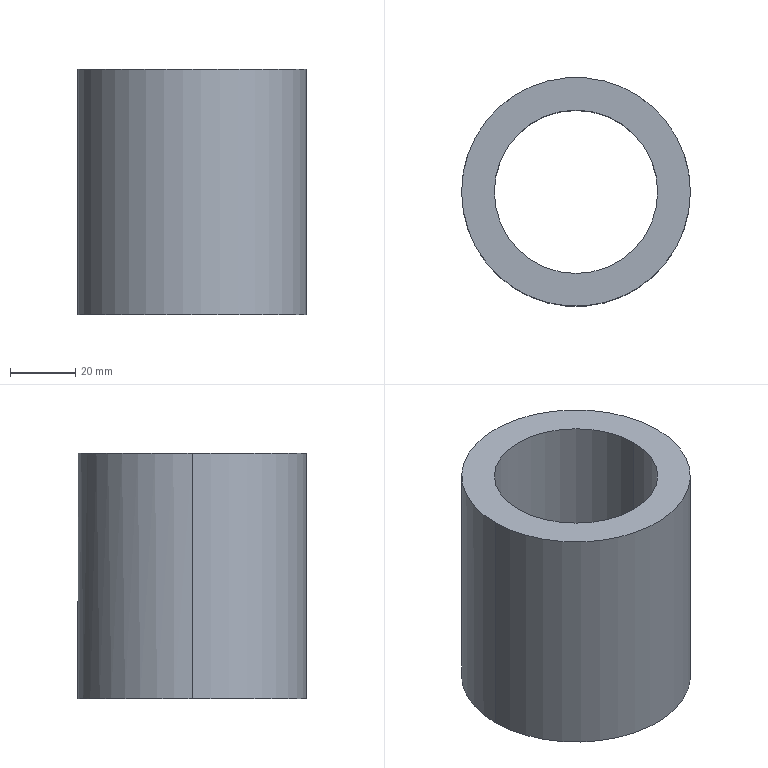Part | Creo | 1 solid | 10 faces | box 70 x 70 x 75 mm | volume 141338 mm3 | cylinder 4 | torus 4 | plane 2 | commonest cylinder face diameters 50 x2 70 x2
STEP:
#1=CARTESIAN_POINT('',(0.,0.,0.));
#2=DIRECTION('',(0.,0.,1.));
#3=DIRECTION('',(1.,0.,0.));
#4=AXIS2_PLACEMENT_3D('',#1,#2,#3);
#5=CARTESIAN_POINT('',(461.101,252.373,51.559));
#6=VERTEX_POINT('',#5);
#7=CARTESIAN_POINT('',(391.101,252.373,51.559));
#8=VERTEX_POINT('',#7);
#9=CARTESIAN_POINT('',(426.101,252.373,51.559));
#10=DIRECTION('',(0.,0.,1.));
#11=DIRECTION('',(1.,0.,0.));
#12=AXIS2_PLACEMENT_3D('',#9,#10,#11);
#13=CIRCLE('',#12,35.);
#14=EDGE_CURVE('',#6,#8,#13,.T.);
#15=ORIENTED_EDGE('',*,*,#14,.F.);
#16=CARTESIAN_POINT('',(426.101,252.373,51.559));
#17=DIRECTION('',(0.,0.,1.));
#18=DIRECTION('',(-1.,0.,0.));
#19=AXIS2_PLACEMENT_3D('',#16,#17,#18);
#20=CIRCLE('',#19,35.);
#21=EDGE_CURVE('',#8,#6,#20,.T.);
#22=ORIENTED_EDGE('',*,*,#21,.F.);
#23=EDGE_LOOP('',(#15,#22));
#24=FACE_OUTER_BOUND('',#23,.F.);
#25=CARTESIAN_POINT('',(451.101,252.373,51.559));
#26=VERTEX_POINT('',#25);
#27=CARTESIAN_POINT('',(401.101,252.373,51.559));
#28=VERTEX_POINT('',#27);
#29=CARTESIAN_POINT('',(426.101,252.373,51.559));
#30=DIRECTION('',(0.,0.,-1.));
#31=DIRECTION('',(1.,0.,0.));
#32=AXIS2_PLACEMENT_3D('',#29,#30,#31);
#33=CIRCLE('',#32,25.);
#34=EDGE_CURVE('',#26,#28,#33,.T.);
#35=ORIENTED_EDGE('',*,*,#34,.F.);
#36=CARTESIAN_POINT('',(426.101,252.373,51.559));
#37=DIRECTION('',(0.,0.,-1.));
#38=DIRECTION('',(-1.,0.,0.));
#39=AXIS2_PLACEMENT_3D('',#36,#37,#38);
#40=CIRCLE('',#39,25.);
#41=EDGE_CURVE('',#28,#26,#40,.T.);
#42=ORIENTED_EDGE('',*,*,#41,.F.);
#43=EDGE_LOOP('',(#35,#42));
#44=FACE_BOUND('',#43,.F.);
#45=CARTESIAN_POINT('',(387.842,227.873,51.559));
#46=DIRECTION('',(0.,0.,1.));
#47=DIRECTION('',(1.,0.,0.));
#48=AXIS2_PLACEMENT_3D('',#45,#46,#47);
#49=PLANE('',#48);
#50=ADVANCED_FACE('',(#24,#44),#49,.T.);
#51=CARTESIAN_POINT('',(391.101,252.373,-23.441));
#52=VERTEX_POINT('',#51);
#53=CARTESIAN_POINT('',(426.101,287.373,-23.441));
#54=VERTEX_POINT('',#53);
#55=CARTESIAN_POINT('',(426.101,252.373,-23.441));
#56=DIRECTION('',(0.,0.,-1.));
#57=DIRECTION('',(-1.,0.,0.));
#58=AXIS2_PLACEMENT_3D('',#55,#56,#57);
#59=CIRCLE('',#58,35.);
#60=EDGE_CURVE('',#52,#54,#59,.T.);
#61=ORIENTED_EDGE('',*,*,#60,.T.);
#62=CARTESIAN_POINT('',(461.101,252.373,-23.441));
#63=VERTEX_POINT('',#62);
#64=CARTESIAN_POINT('',(426.101,252.373,-23.441));
#65=DIRECTION('',(0.,0.,-1.));
#66=DIRECTION('',(0.,1.,0.));
#67=AXIS2_PLACEMENT_3D('',#64,#65,#66);
#68=CIRCLE('',#67,35.);
#69=EDGE_CURVE('',#54,#63,#68,.T.);
#70=ORIENTED_EDGE('',*,*,#69,.T.);
#71=CARTESIAN_POINT('',(461.101,252.373,-23.441));
#72=DIRECTION('',(0.,0.,1.));
#73=VECTOR('',#72,75.);
#74=LINE('',#71,#73);
#75=EDGE_CURVE('',#63,#6,#74,.T.);
#76=ORIENTED_EDGE('',*,*,#75,.T.);
#77=ORIENTED_EDGE('',*,*,#14,.T.);
#78=CARTESIAN_POINT('',(391.101,252.373,-23.441));
#79=DIRECTION('',(0.,0.,1.));
#80=VECTOR('',#79,75.);
#81=LINE('',#78,#80);
#82=EDGE_CURVE('',#52,#8,#81,.T.);
#83=ORIENTED_EDGE('',*,*,#82,.F.);
#84=EDGE_LOOP('',(#61,#70,#76,#77,#83));
#85=FACE_OUTER_BOUND('',#84,.F.);
#86=CARTESIAN_POINT('',(426.101,252.373,-23.441));
#87=DIRECTION('',(0.,0.,1.));
#88=DIRECTION('',(1.,0.,0.));
#89=AXIS2_PLACEMENT_3D('',#86,#87,#88);
#90=CYLINDRICAL_SURFACE('',#89,35.);
#91=ADVANCED_FACE('',(#85),#90,.T.);
#92=ORIENTED_EDGE('',*,*,#69,.F.);
#93=ORIENTED_EDGE('',*,*,#60,.F.);
#94=CARTESIAN_POINT('',(426.101,252.373,-23.441));
#95=DIRECTION('',(0.,0.,-1.));
#96=DIRECTION('',(1.,0.,0.));
#97=AXIS2_PLACEMENT_3D('',#94,#95,#96);
#98=CIRCLE('',#97,35.);
#99=EDGE_CURVE('',#63,#52,#98,.T.);
#100=ORIENTED_EDGE('',*,*,#99,.F.);
#101=EDGE_LOOP('',(#92,#93,#100));
#102=FACE_OUTER_BOUND('',#101,.F.);
#103=CARTESIAN_POINT('',(426.101,278.373,-23.441));
#104=VERTEX_POINT('',#103);
#105=CARTESIAN_POINT('',(400.101,252.373,-23.441));
#106=VERTEX_POINT('',#105);
#107=CARTESIAN_POINT('',(426.101,252.373,-23.441));
#108=DIRECTION('',(0.,0.,1.));
#109=DIRECTION('',(0.,1.,0.));
#110=AXIS2_PLACEMENT_3D('',#107,#108,#109);
#111=CIRCLE('',#110,26.);
#112=EDGE_CURVE('',#104,#106,#111,.T.);
#113=ORIENTED_EDGE('',*,*,#112,.F.);
#114=CARTESIAN_POINT('',(452.101,252.373,-23.441));
#115=VERTEX_POINT('',#114);
#116=CARTESIAN_POINT('',(426.101,252.373,-23.441));
#117=DIRECTION('',(0.,0.,1.));
#118=DIRECTION('',(1.,0.,0.));
#119=AXIS2_PLACEMENT_3D('',#116,#117,#118);
#120=CIRCLE('',#119,26.);
#121=EDGE_CURVE('',#115,#104,#120,.T.);
#122=ORIENTED_EDGE('',*,*,#121,.F.);
#123=CARTESIAN_POINT('',(426.101,226.373,-23.441));
#124=VERTEX_POINT('',#123);
#125=CARTESIAN_POINT('',(426.101,252.373,-23.441));
#126=DIRECTION('',(0.,0.,1.));
#127=DIRECTION('',(0.,-1.,0.));
#128=AXIS2_PLACEMENT_3D('',#125,#126,#127);
#129=CIRCLE('',#128,26.);
#130=EDGE_CURVE('',#124,#115,#129,.T.);
#131=ORIENTED_EDGE('',*,*,#130,.F.);
#132=CARTESIAN_POINT('',(426.101,252.373,-23.441));
#133=DIRECTION('',(0.,0.,1.));
#134=DIRECTION('',(-1.,0.,0.));
#135=AXIS2_PLACEMENT_3D('',#132,#133,#134);
#136=CIRCLE('',#135,26.);
#137=EDGE_CURVE('',#106,#124,#136,.T.);
#138=ORIENTED_EDGE('',*,*,#137,.F.);
#139=EDGE_LOOP('',(#113,#122,#131,#138));
#140=FACE_BOUND('',#139,.F.);
#141=CARTESIAN_POINT('',(426.101,252.373,-23.441));
#142=DIRECTION('',(0.,0.,1.));
#143=DIRECTION('',(1.,0.,0.));
#144=AXIS2_PLACEMENT_3D('',#141,#142,#143);
#145=PLANE('',#144);
#146=ADVANCED_FACE('',(#102,#140),#145,.F.);
#147=ORIENTED_EDGE('',*,*,#121,.T.);
#148=ORIENTED_EDGE('',*,*,#112,.T.);
#149=CARTESIAN_POINT('',(400.808,252.373,-23.149));
#150=VERTEX_POINT('',#149);
#151=CARTESIAN_POINT('',(400.101,252.373,-22.441));
#152=DIRECTION('',(0.,1.,0.));
#153=DIRECTION('',(0.7071,0.,-0.7071));
#154=AXIS2_PLACEMENT_3D('',#151,#152,#153);
#155=CIRCLE('',#154,1.);
#156=EDGE_CURVE('',#150,#106,#155,.T.);
#157=ORIENTED_EDGE('',*,*,#156,.F.);
#158=CARTESIAN_POINT('',(451.394,252.373,-23.149));
#159=VERTEX_POINT('',#158);
#160=CARTESIAN_POINT('',(426.101,252.373,-23.149));
#161=DIRECTION('',(0.,0.,1.));
#162=DIRECTION('',(1.,0.,0.));
#163=AXIS2_PLACEMENT_3D('',#160,#161,#162);
#164=CIRCLE('',#163,25.293);
#165=EDGE_CURVE('',#159,#150,#164,.T.);
#166=ORIENTED_EDGE('',*,*,#165,.F.);
#167=CARTESIAN_POINT('',(452.101,252.373,-22.441));
#168=DIRECTION('',(0.,-1.,0.));
#169=DIRECTION('',(-0.7071,0.,-0.7071));
#170=AXIS2_PLACEMENT_3D('',#167,#168,#169);
#171=CIRCLE('',#170,1.);
#172=EDGE_CURVE('',#159,#115,#171,.T.);
#173=ORIENTED_EDGE('',*,*,#172,.T.);
#174=EDGE_LOOP('',(#147,#148,#157,#166,#173));
#175=FACE_OUTER_BOUND('',#174,.F.);
#176=CARTESIAN_POINT('',(426.101,252.373,-22.441));
#177=DIRECTION('',(0.,0.,1.));
#178=DIRECTION('',(1.,0.,0.));
#179=AXIS2_PLACEMENT_3D('',#176,#177,#178);
#180=TOROIDAL_SURFACE('',#179,26.,1.);
#181=ADVANCED_FACE('',(#175),#180,.T.);
#182=ORIENTED_EDGE('',*,*,#130,.T.);
#183=ORIENTED_EDGE('',*,*,#172,.F.);
#184=CARTESIAN_POINT('',(426.101,252.373,-23.149));
#185=DIRECTION('',(0.,0.,1.));
#186=DIRECTION('',(-1.,0.,0.));
#187=AXIS2_PLACEMENT_3D('',#184,#185,#186);
#188=CIRCLE('',#187,25.293);
#189=EDGE_CURVE('',#150,#159,#188,.T.);
#190=ORIENTED_EDGE('',*,*,#189,.F.);
#191=ORIENTED_EDGE('',*,*,#156,.T.);
#192=ORIENTED_EDGE('',*,*,#137,.T.);
#193=EDGE_LOOP('',(#182,#183,#190,#191,#192));
#194=FACE_OUTER_BOUND('',#193,.F.);
#195=CARTESIAN_POINT('',(426.101,252.373,-22.441));
#196=DIRECTION('',(0.,0.,1.));
#197=DIRECTION('',(1.,0.,0.));
#198=AXIS2_PLACEMENT_3D('',#195,#196,#197);
#199=TOROIDAL_SURFACE('',#198,26.,1.);
#200=ADVANCED_FACE('',(#194),#199,.T.);
#201=CARTESIAN_POINT('',(401.101,252.373,-22.441));
#202=VERTEX_POINT('',#201);
#203=CARTESIAN_POINT('',(451.101,252.373,-22.441));
#204=VERTEX_POINT('',#203);
#205=CARTESIAN_POINT('',(426.101,252.373,-22.441));
#206=DIRECTION('',(0.,0.,1.));
#207=DIRECTION('',(-1.,0.,0.));
#208=AXIS2_PLACEMENT_3D('',#205,#206,#207);
#209=CIRCLE('',#208,25.);
#210=EDGE_CURVE('',#202,#204,#209,.T.);
#211=ORIENTED_EDGE('',*,*,#210,.F.);
#212=CARTESIAN_POINT('',(400.101,252.373,-22.441));
#213=DIRECTION('',(0.,1.,0.));
#214=DIRECTION('',(1.,0.,0.));
#215=AXIS2_PLACEMENT_3D('',#212,#213,#214);
#216=CIRCLE('',#215,1.);
#217=EDGE_CURVE('',#202,#150,#216,.T.);
#218=ORIENTED_EDGE('',*,*,#217,.T.);
#219=ORIENTED_EDGE('',*,*,#189,.T.);
#220=CARTESIAN_POINT('',(452.101,252.373,-22.441));
#221=DIRECTION('',(0.,-1.,0.));
#222=DIRECTION('',(-1.,0.,0.));
#223=AXIS2_PLACEMENT_3D('',#220,#221,#222);
#224=CIRCLE('',#223,1.);
#225=EDGE_CURVE('',#204,#159,#224,.T.);
#226=ORIENTED_EDGE('',*,*,#225,.F.);
#227=EDGE_LOOP('',(#211,#218,#219,#226));
#228=FACE_OUTER_BOUND('',#227,.F.);
#229=CARTESIAN_POINT('',(426.101,252.373,-22.441));
#230=DIRECTION('',(0.,0.,1.));
#231=DIRECTION('',(1.,0.,0.));
#232=AXIS2_PLACEMENT_3D('',#229,#230,#231);
#233=TOROIDAL_SURFACE('',#232,26.,1.);
#234=ADVANCED_FACE('',(#228),#233,.T.);
#235=ORIENTED_EDGE('',*,*,#210,.T.);
#236=CARTESIAN_POINT('',(451.101,252.373,-22.441));
#237=DIRECTION('',(0.,0.,1.));
#238=VECTOR('',#237,74.);
#239=LINE('',#236,#238);
#240=EDGE_CURVE('',#204,#26,#239,.T.);
#241=ORIENTED_EDGE('',*,*,#240,.T.);
#242=ORIENTED_EDGE('',*,*,#34,.T.);
#243=CARTESIAN_POINT('',(401.101,252.373,-22.441));
#244=DIRECTION('',(0.,0.,1.));
#245=VECTOR('',#244,74.);
#246=LINE('',#243,#245);
#247=EDGE_CURVE('',#202,#28,#246,.T.);
#248=ORIENTED_EDGE('',*,*,#247,.F.);
#249=EDGE_LOOP('',(#235,#241,#242,#248));
#250=FACE_OUTER_BOUND('',#249,.F.);
#251=CARTESIAN_POINT('',(426.101,252.373,-23.441));
#252=DIRECTION('',(0.,0.,1.));
#253=DIRECTION('',(1.,0.,0.));
#254=AXIS2_PLACEMENT_3D('',#251,#252,#253);
#255=CYLINDRICAL_SURFACE('',#254,25.);
#256=ADVANCED_FACE('',(#250),#255,.F.);
#257=CARTESIAN_POINT('',(426.101,277.373,-22.441));
#258=VERTEX_POINT('',#257);
#259=CARTESIAN_POINT('',(426.101,252.373,-22.441));
#260=DIRECTION('',(0.,0.,1.));
#261=DIRECTION('',(1.,0.,0.));
#262=AXIS2_PLACEMENT_3D('',#259,#260,#261);
#263=CIRCLE('',#262,25.);
#264=EDGE_CURVE('',#204,#258,#263,.T.);
#265=ORIENTED_EDGE('',*,*,#264,.T.);
#266=CARTESIAN_POINT('',(426.101,252.373,-22.441));
#267=DIRECTION('',(0.,0.,1.));
#268=DIRECTION('',(0.,1.,0.));
#269=AXIS2_PLACEMENT_3D('',#266,#267,#268);
#270=CIRCLE('',#269,25.);
#271=EDGE_CURVE('',#258,#202,#270,.T.);
#272=ORIENTED_EDGE('',*,*,#271,.T.);
#273=ORIENTED_EDGE('',*,*,#247,.T.);
#274=ORIENTED_EDGE('',*,*,#41,.T.);
#275=ORIENTED_EDGE('',*,*,#240,.F.);
#276=EDGE_LOOP('',(#265,#272,#273,#274,#275));
#277=FACE_OUTER_BOUND('',#276,.F.);
#278=CARTESIAN_POINT('',(426.101,252.373,-23.441));
#279=DIRECTION('',(0.,0.,1.));
#280=DIRECTION('',(1.,0.,0.));
#281=AXIS2_PLACEMENT_3D('',#278,#279,#280);
#282=CYLINDRICAL_SURFACE('',#281,25.);
#283=ADVANCED_FACE('',(#277),#282,.F.);
#284=ORIENTED_EDGE('',*,*,#271,.F.);
#285=ORIENTED_EDGE('',*,*,#264,.F.);
#286=ORIENTED_EDGE('',*,*,#225,.T.);
#287=ORIENTED_EDGE('',*,*,#165,.T.);
#288=ORIENTED_EDGE('',*,*,#217,.F.);
#289=EDGE_LOOP('',(#284,#285,#286,#287,#288));
#290=FACE_OUTER_BOUND('',#289,.F.);
#291=CARTESIAN_POINT('',(426.101,252.373,-22.441));
#292=DIRECTION('',(0.,0.,1.));
#293=DIRECTION('',(1.,0.,0.));
#294=AXIS2_PLACEMENT_3D('',#291,#292,#293);
#295=TOROIDAL_SURFACE('',#294,26.,1.);
#296=ADVANCED_FACE('',(#290),#295,.T.);
#297=ORIENTED_EDGE('',*,*,#99,.T.);
#298=ORIENTED_EDGE('',*,*,#82,.T.);
#299=ORIENTED_EDGE('',*,*,#21,.T.);
#300=ORIENTED_EDGE('',*,*,#75,.F.);
#301=EDGE_LOOP('',(#297,#298,#299,#300));
#302=FACE_OUTER_BOUND('',#301,.F.);
#303=CARTESIAN_POINT('',(426.101,252.373,-23.441));
#304=DIRECTION('',(0.,0.,1.));
#305=DIRECTION('',(1.,0.,0.));
#306=AXIS2_PLACEMENT_3D('',#303,#304,#305);
#307=CYLINDRICAL_SURFACE('',#306,35.);
#308=ADVANCED_FACE('',(#302),#307,.T.);
#309=CLOSED_SHELL('',(#50,#91,#146,#181,#200,#234,#256,#283,#296,#308));
#310=MANIFOLD_SOLID_BREP('',#309);
#311=(LENGTH_UNIT()NAMED_UNIT(*)SI_UNIT(.MILLI.,.METRE.));
#312=UNCERTAINTY_MEASURE_WITH_UNIT(LENGTH_MEASURE(0.01242),#311,'','');
#313=(NAMED_UNIT(*)PLANE_ANGLE_UNIT()SI_UNIT($,.RADIAN.));
#314=PLANE_ANGLE_MEASURE_WITH_UNIT(PLANE_ANGLE_MEASURE(0.01745),#313);
#315=(CONVERSION_BASED_UNIT('DEGREE',#314)NAMED_UNIT(*)PLANE_ANGLE_UNIT());
#316=(NAMED_UNIT(*)SI_UNIT($,.STERADIAN.)SOLID_ANGLE_UNIT());
#317=(GEOMETRIC_REPRESENTATION_CONTEXT(3)GLOBAL_UNCERTAINTY_ASSIGNED_CONTEXT((#312))GLOBAL_UNIT_ASSIGNED_CONTEXT((#311,#315,#316))REPRESENTATION_CONTEXT('',''));
#318=ADVANCED_BREP_SHAPE_REPRESENTATION('',(#4,#310),#317);